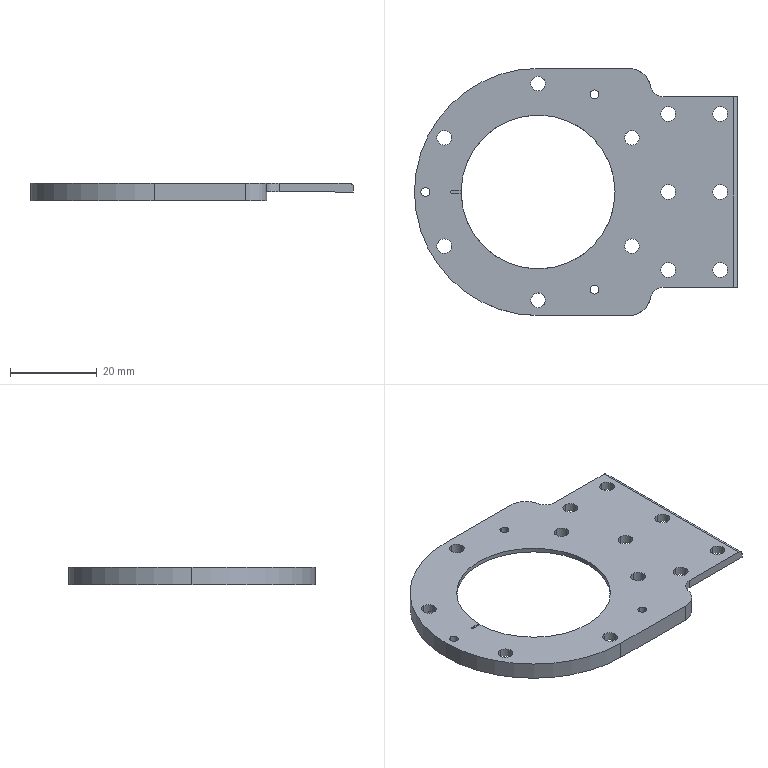Part | 1 solid | 76 faces | box 74.5 x 57 x 4 mm | volume 6653 mm3 | cylinder 62 | plane 14 | commonest cylinder face diameters 3.4 x24 2 x15 2.05 x6 47 x6 6 x2 10 x2